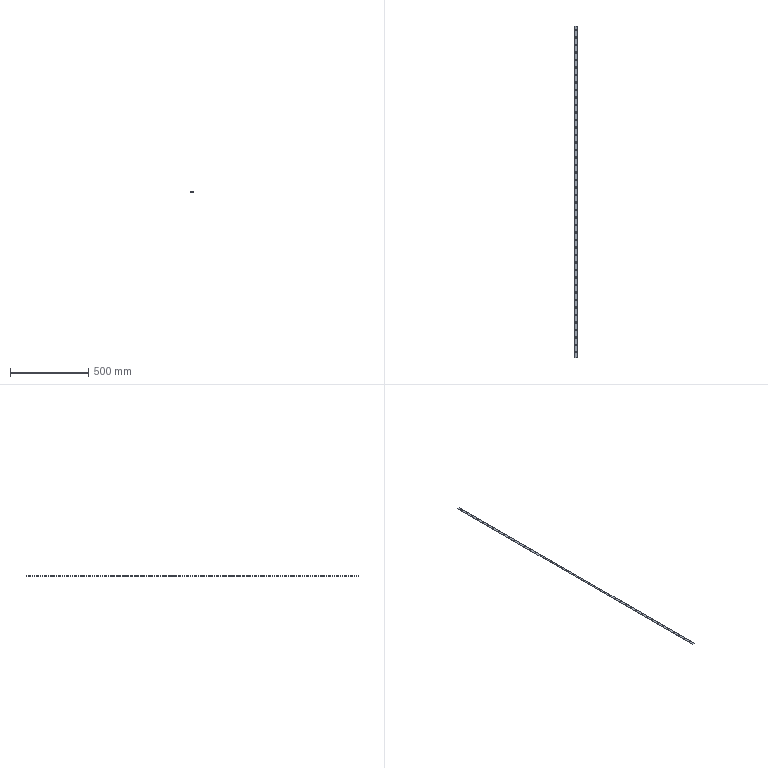Part | NX | features solid 2 | 1 solid | 94 faces | box 16 x 2126 x 0.54 mm | volume 17174 mm3 | cylinder 88 | plane 6 | commonest cylinder face diameters 8 x88